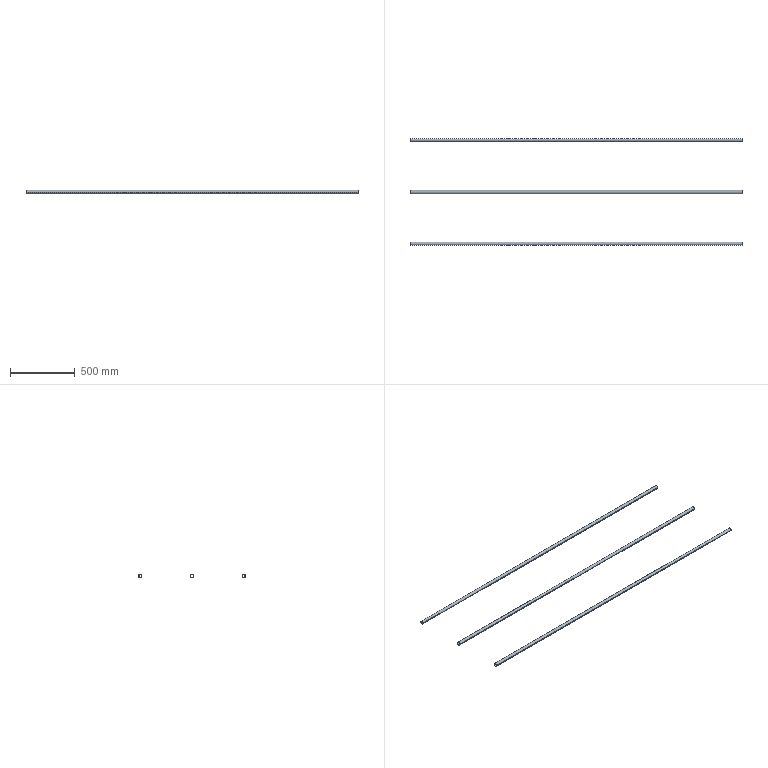Part | STEP file | E3-中转釜护栏2栏杆_Default<As Machined> | 3 solids | 18 faces | box 2560 x 825 x 25 mm | volume 850492 mm3 | cylinder 12 | plane 6 | commonest cylinder face diameters 22 x6 25 x6
STEP:
#1=CARTESIAN_POINT('',(0.,0.,0.));
#2=DIRECTION('',(0.,0.,1.));
#3=DIRECTION('',(1.,0.,0.));
#4=AXIS2_PLACEMENT_3D('',#1,#2,#3);
#5=CARTESIAN_POINT('',(1280.,787.5,0.));
#6=VERTEX_POINT('',#5);
#7=CARTESIAN_POINT('',(1280.,812.5,0.));
#8=VERTEX_POINT('',#7);
#9=CARTESIAN_POINT('',(1280.,800.,0.));
#10=DIRECTION('',(-1.,0.,0.));
#11=DIRECTION('',(0.,1.,0.));
#12=AXIS2_PLACEMENT_3D('',#9,#10,#11);
#13=CIRCLE('',#12,12.5);
#14=CARTESIAN_POINT('',(1280.,800.,0.));
#15=DIRECTION('',(-1.,0.,0.));
#16=DIRECTION('',(0.,-1.,0.));
#17=AXIS2_PLACEMENT_3D('',#14,#15,#16);
#18=CYLINDRICAL_SURFACE('',#17,12.5);
#19=CARTESIAN_POINT('',(-3.142,0.));
#20=DIRECTION('',(1.,0.));
#21=VECTOR('',#20,1.);
#22=LINE('',#19,#21);
#23=(GEOMETRIC_REPRESENTATION_CONTEXT(2)PARAMETRIC_REPRESENTATION_CONTEXT()REPRESENTATION_CONTEXT('',''));
#24=DEFINITIONAL_REPRESENTATION('',(#22),#23);
#25=PCURVE('',#18,#24);
#26=CARTESIAN_POINT('',(1280.,800.,0.));
#27=DIRECTION('',(1.,0.,0.));
#28=DIRECTION('',(0.,1.,0.));
#29=AXIS2_PLACEMENT_3D('',#26,#27,#28);
#30=PLANE('',#29);
#31=CARTESIAN_POINT('',(12.5,0.));
#32=CARTESIAN_POINT('',(12.5,-21.651));
#33=CARTESIAN_POINT('',(-6.25,-10.825));
#34=CARTESIAN_POINT('',(-25.,0.));
#35=CARTESIAN_POINT('',(-6.25,10.825));
#36=CARTESIAN_POINT('',(12.5,21.651));
#37=CARTESIAN_POINT('',(12.5,0.));
#38=(BOUNDED_CURVE()B_SPLINE_CURVE(2,(#31,#32,#33,#34,#35,#36,#37),.UNSPECIFIED.,.T.,.F.)B_SPLINE_CURVE_WITH_KNOTS((1,2,2,2,2,1),(-2.094,0.,2.094,4.189,6.283,8.378),.UNSPECIFIED.)CURVE()GEOMETRIC_REPRESENTATION_ITEM()RATIONAL_B_SPLINE_CURVE((1.,0.5,1.,0.5,1.,0.5,1.))REPRESENTATION_ITEM(''));
#39=(GEOMETRIC_REPRESENTATION_CONTEXT(2)PARAMETRIC_REPRESENTATION_CONTEXT()REPRESENTATION_CONTEXT('',''));
#40=DEFINITIONAL_REPRESENTATION('',(#38),#39);
#41=PCURVE('',#30,#40);
#42=SURFACE_CURVE('',#13,(#25,#41),.PCURVE_S1.);
#43=EDGE_CURVE('',#6,#8,#42,.T.);
#44=ORIENTED_EDGE('',*,*,#43,.T.);
#45=CARTESIAN_POINT('',(-1280.,812.5,0.));
#46=VERTEX_POINT('',#45);
#47=CARTESIAN_POINT('',(1280.,812.5,0.));
#48=DIRECTION('',(-1.,0.,0.));
#49=VECTOR('',#48,1.);
#50=LINE('',#47,#49);
#51=CARTESIAN_POINT('',(3.142,0.));
#52=DIRECTION('',(0.,1.));
#53=VECTOR('',#52,1.);
#54=LINE('',#51,#53);
#55=(GEOMETRIC_REPRESENTATION_CONTEXT(2)PARAMETRIC_REPRESENTATION_CONTEXT()REPRESENTATION_CONTEXT('',''));
#56=DEFINITIONAL_REPRESENTATION('',(#54),#55);
#57=PCURVE('',#18,#56);
#58=CARTESIAN_POINT('',(1280.,800.,0.));
#59=DIRECTION('',(-1.,0.,0.));
#60=DIRECTION('',(0.,-1.,0.));
#61=AXIS2_PLACEMENT_3D('',#58,#59,#60);
#62=CYLINDRICAL_SURFACE('',#61,12.5);
#63=CARTESIAN_POINT('',(3.142,0.));
#64=DIRECTION('',(0.,1.));
#65=VECTOR('',#64,1.);
#66=LINE('',#63,#65);
#67=(GEOMETRIC_REPRESENTATION_CONTEXT(2)PARAMETRIC_REPRESENTATION_CONTEXT()REPRESENTATION_CONTEXT('',''));
#68=DEFINITIONAL_REPRESENTATION('',(#66),#67);
#69=PCURVE('',#62,#68);
#70=SURFACE_CURVE('',#50,(#57,#69),.PCURVE_S1.);
#71=EDGE_CURVE('',#8,#46,#70,.T.);
#72=ORIENTED_EDGE('',*,*,#71,.T.);
#73=CARTESIAN_POINT('',(-1280.,787.5,0.));
#74=VERTEX_POINT('',#73);
#75=CARTESIAN_POINT('',(-1280.,800.,0.));
#76=DIRECTION('',(-1.,0.,0.));
#77=DIRECTION('',(0.,1.,0.));
#78=AXIS2_PLACEMENT_3D('',#75,#76,#77);
#79=CIRCLE('',#78,12.5);
#80=CARTESIAN_POINT('',(-3.142,2560.));
#81=DIRECTION('',(1.,0.));
#82=VECTOR('',#81,1.);
#83=LINE('',#80,#82);
#84=(GEOMETRIC_REPRESENTATION_CONTEXT(2)PARAMETRIC_REPRESENTATION_CONTEXT()REPRESENTATION_CONTEXT('',''));
#85=DEFINITIONAL_REPRESENTATION('',(#83),#84);
#86=PCURVE('',#18,#85);
#87=CARTESIAN_POINT('',(-1280.,800.,0.));
#88=DIRECTION('',(1.,0.,0.));
#89=DIRECTION('',(0.,1.,0.));
#90=AXIS2_PLACEMENT_3D('',#87,#88,#89);
#91=PLANE('',#90);
#92=CARTESIAN_POINT('',(12.5,0.));
#93=CARTESIAN_POINT('',(12.5,-21.651));
#94=CARTESIAN_POINT('',(-6.25,-10.825));
#95=CARTESIAN_POINT('',(-25.,0.));
#96=CARTESIAN_POINT('',(-6.25,10.825));
#97=CARTESIAN_POINT('',(12.5,21.651));
#98=CARTESIAN_POINT('',(12.5,0.));
#99=(BOUNDED_CURVE()B_SPLINE_CURVE(2,(#92,#93,#94,#95,#96,#97,#98),.UNSPECIFIED.,.T.,.F.)B_SPLINE_CURVE_WITH_KNOTS((1,2,2,2,2,1),(-2.094,0.,2.094,4.189,6.283,8.378),.UNSPECIFIED.)CURVE()GEOMETRIC_REPRESENTATION_ITEM()RATIONAL_B_SPLINE_CURVE((1.,0.5,1.,0.5,1.,0.5,1.))REPRESENTATION_ITEM(''));
#100=(GEOMETRIC_REPRESENTATION_CONTEXT(2)PARAMETRIC_REPRESENTATION_CONTEXT()REPRESENTATION_CONTEXT('',''));
#101=DEFINITIONAL_REPRESENTATION('',(#99),#100);
#102=PCURVE('',#91,#101);
#103=SURFACE_CURVE('',#79,(#86,#102),.PCURVE_S1.);
#104=EDGE_CURVE('',#74,#46,#103,.T.);
#105=ORIENTED_EDGE('',*,*,#104,.F.);
#106=CARTESIAN_POINT('',(1280.,787.5,0.));
#107=DIRECTION('',(-1.,0.,0.));
#108=VECTOR('',#107,1.);
#109=LINE('',#106,#108);
#110=CARTESIAN_POINT('',(0.,0.));
#111=DIRECTION('',(0.,1.));
#112=VECTOR('',#111,1.);
#113=LINE('',#110,#112);
#114=(GEOMETRIC_REPRESENTATION_CONTEXT(2)PARAMETRIC_REPRESENTATION_CONTEXT()REPRESENTATION_CONTEXT('',''));
#115=DEFINITIONAL_REPRESENTATION('',(#113),#114);
#116=PCURVE('',#18,#115);
#117=CARTESIAN_POINT('',(6.283,0.));
#118=DIRECTION('',(0.,1.));
#119=VECTOR('',#118,1.);
#120=LINE('',#117,#119);
#121=(GEOMETRIC_REPRESENTATION_CONTEXT(2)PARAMETRIC_REPRESENTATION_CONTEXT()REPRESENTATION_CONTEXT('',''));
#122=DEFINITIONAL_REPRESENTATION('',(#120),#121);
#123=PCURVE('',#62,#122);
#124=SURFACE_CURVE('',#109,(#116,#123),.PCURVE_S1.);
#125=EDGE_CURVE('',#6,#74,#124,.T.);
#126=ORIENTED_EDGE('',*,*,#125,.F.);
#127=EDGE_LOOP('',(#44,#72,#105,#126));
#128=FACE_BOUND('',#127,.T.);
#129=ADVANCED_FACE('',(#128),#18,.T.);
#130=CARTESIAN_POINT('',(1280.,789.,0.));
#131=VERTEX_POINT('',#130);
#132=CARTESIAN_POINT('',(-1280.,789.,0.));
#133=VERTEX_POINT('',#132);
#134=CARTESIAN_POINT('',(1280.,789.,0.));
#135=DIRECTION('',(-1.,0.,0.));
#136=VECTOR('',#135,1.);
#137=LINE('',#134,#136);
#138=CARTESIAN_POINT('',(1280.,800.,0.));
#139=DIRECTION('',(-1.,0.,0.));
#140=DIRECTION('',(0.,-1.,0.));
#141=AXIS2_PLACEMENT_3D('',#138,#139,#140);
#142=CYLINDRICAL_SURFACE('',#141,11.);
#143=CARTESIAN_POINT('',(6.283,0.));
#144=DIRECTION('',(0.,1.));
#145=VECTOR('',#144,1.);
#146=LINE('',#143,#145);
#147=(GEOMETRIC_REPRESENTATION_CONTEXT(2)PARAMETRIC_REPRESENTATION_CONTEXT()REPRESENTATION_CONTEXT('',''));
#148=DEFINITIONAL_REPRESENTATION('',(#146),#147);
#149=PCURVE('',#142,#148);
#150=CARTESIAN_POINT('',(1280.,800.,0.));
#151=DIRECTION('',(-1.,0.,0.));
#152=DIRECTION('',(0.,-1.,0.));
#153=AXIS2_PLACEMENT_3D('',#150,#151,#152);
#154=CYLINDRICAL_SURFACE('',#153,11.);
#155=CARTESIAN_POINT('',(0.,0.));
#156=DIRECTION('',(0.,1.));
#157=VECTOR('',#156,1.);
#158=LINE('',#155,#157);
#159=(GEOMETRIC_REPRESENTATION_CONTEXT(2)PARAMETRIC_REPRESENTATION_CONTEXT()REPRESENTATION_CONTEXT('',''));
#160=DEFINITIONAL_REPRESENTATION('',(#158),#159);
#161=PCURVE('',#154,#160);
#162=SURFACE_CURVE('',#137,(#149,#161),.PCURVE_S1.);
#163=EDGE_CURVE('',#131,#133,#162,.T.);
#164=ORIENTED_EDGE('',*,*,#163,.T.);
#165=CARTESIAN_POINT('',(-1280.,811.,0.));
#166=VERTEX_POINT('',#165);
#167=CARTESIAN_POINT('',(-1280.,800.,0.));
#168=DIRECTION('',(-1.,0.,0.));
#169=DIRECTION('',(0.,1.,0.));
#170=AXIS2_PLACEMENT_3D('',#167,#168,#169);
#171=CIRCLE('',#170,11.);
#172=CARTESIAN_POINT('',(3.142,2560.));
#173=DIRECTION('',(1.,0.));
#174=VECTOR('',#173,1.);
#175=LINE('',#172,#174);
#176=(GEOMETRIC_REPRESENTATION_CONTEXT(2)PARAMETRIC_REPRESENTATION_CONTEXT()REPRESENTATION_CONTEXT('',''));
#177=DEFINITIONAL_REPRESENTATION('',(#175),#176);
#178=PCURVE('',#142,#177);
#179=CARTESIAN_POINT('',(11.,0.));
#180=CARTESIAN_POINT('',(11.,-19.053));
#181=CARTESIAN_POINT('',(-5.5,-9.526));
#182=CARTESIAN_POINT('',(-22.,0.));
#183=CARTESIAN_POINT('',(-5.5,9.526));
#184=CARTESIAN_POINT('',(11.,19.053));
#185=CARTESIAN_POINT('',(11.,0.));
#186=(BOUNDED_CURVE()B_SPLINE_CURVE(2,(#179,#180,#181,#182,#183,#184,#185),.UNSPECIFIED.,.T.,.F.)B_SPLINE_CURVE_WITH_KNOTS((1,2,2,2,2,1),(-2.094,0.,2.094,4.189,6.283,8.378),.UNSPECIFIED.)CURVE()GEOMETRIC_REPRESENTATION_ITEM()RATIONAL_B_SPLINE_CURVE((1.,0.5,1.,0.5,1.,0.5,1.))REPRESENTATION_ITEM(''));
#187=(GEOMETRIC_REPRESENTATION_CONTEXT(2)PARAMETRIC_REPRESENTATION_CONTEXT()REPRESENTATION_CONTEXT('',''));
#188=DEFINITIONAL_REPRESENTATION('',(#186),#187);
#189=PCURVE('',#91,#188);
#190=SURFACE_CURVE('',#171,(#178,#189),.PCURVE_S1.);
#191=EDGE_CURVE('',#166,#133,#190,.T.);
#192=ORIENTED_EDGE('',*,*,#191,.F.);
#193=CARTESIAN_POINT('',(1280.,811.,0.));
#194=VERTEX_POINT('',#193);
#195=CARTESIAN_POINT('',(1280.,811.,0.));
#196=DIRECTION('',(-1.,0.,0.));
#197=VECTOR('',#196,1.);
#198=LINE('',#195,#197);
#199=CARTESIAN_POINT('',(3.142,0.));
#200=DIRECTION('',(0.,1.));
#201=VECTOR('',#200,1.);
#202=LINE('',#199,#201);
#203=(GEOMETRIC_REPRESENTATION_CONTEXT(2)PARAMETRIC_REPRESENTATION_CONTEXT()REPRESENTATION_CONTEXT('',''));
#204=DEFINITIONAL_REPRESENTATION('',(#202),#203);
#205=PCURVE('',#142,#204);
#206=CARTESIAN_POINT('',(3.142,0.));
#207=DIRECTION('',(0.,1.));
#208=VECTOR('',#207,1.);
#209=LINE('',#206,#208);
#210=(GEOMETRIC_REPRESENTATION_CONTEXT(2)PARAMETRIC_REPRESENTATION_CONTEXT()REPRESENTATION_CONTEXT('',''));
#211=DEFINITIONAL_REPRESENTATION('',(#209),#210);
#212=PCURVE('',#154,#211);
#213=SURFACE_CURVE('',#198,(#205,#212),.PCURVE_S1.);
#214=EDGE_CURVE('',#194,#166,#213,.T.);
#215=ORIENTED_EDGE('',*,*,#214,.F.);
#216=CARTESIAN_POINT('',(1280.,800.,0.));
#217=DIRECTION('',(-1.,0.,0.));
#218=DIRECTION('',(0.,1.,0.));
#219=AXIS2_PLACEMENT_3D('',#216,#217,#218);
#220=CIRCLE('',#219,11.);
#221=CARTESIAN_POINT('',(3.142,0.));
#222=DIRECTION('',(1.,0.));
#223=VECTOR('',#222,1.);
#224=LINE('',#221,#223);
#225=(GEOMETRIC_REPRESENTATION_CONTEXT(2)PARAMETRIC_REPRESENTATION_CONTEXT()REPRESENTATION_CONTEXT('',''));
#226=DEFINITIONAL_REPRESENTATION('',(#224),#225);
#227=PCURVE('',#142,#226);
#228=CARTESIAN_POINT('',(11.,0.));
#229=CARTESIAN_POINT('',(11.,-19.053));
#230=CARTESIAN_POINT('',(-5.5,-9.526));
#231=CARTESIAN_POINT('',(-22.,0.));
#232=CARTESIAN_POINT('',(-5.5,9.526));
#233=CARTESIAN_POINT('',(11.,19.053));
#234=CARTESIAN_POINT('',(11.,0.));
#235=(BOUNDED_CURVE()B_SPLINE_CURVE(2,(#228,#229,#230,#231,#232,#233,#234),.UNSPECIFIED.,.T.,.F.)B_SPLINE_CURVE_WITH_KNOTS((1,2,2,2,2,1),(-2.094,0.,2.094,4.189,6.283,8.378),.UNSPECIFIED.)CURVE()GEOMETRIC_REPRESENTATION_ITEM()RATIONAL_B_SPLINE_CURVE((1.,0.5,1.,0.5,1.,0.5,1.))REPRESENTATION_ITEM(''));
#236=(GEOMETRIC_REPRESENTATION_CONTEXT(2)PARAMETRIC_REPRESENTATION_CONTEXT()REPRESENTATION_CONTEXT('',''));
#237=DEFINITIONAL_REPRESENTATION('',(#235),#236);
#238=PCURVE('',#30,#237);
#239=SURFACE_CURVE('',#220,(#227,#238),.PCURVE_S1.);
#240=EDGE_CURVE('',#194,#131,#239,.T.);
#241=ORIENTED_EDGE('',*,*,#240,.T.);
#242=EDGE_LOOP('',(#164,#192,#215,#241));
#243=FACE_BOUND('',#242,.F.);
#244=ADVANCED_FACE('',(#243),#142,.F.);
#245=CARTESIAN_POINT('',(-1280.,800.,0.));
#246=DIRECTION('',(-1.,0.,0.));
#247=DIRECTION('',(0.,1.,0.));
#248=AXIS2_PLACEMENT_3D('',#245,#246,#247);
#249=CIRCLE('',#248,11.);
#250=CARTESIAN_POINT('',(-3.142,2560.));
#251=DIRECTION('',(1.,0.));
#252=VECTOR('',#251,1.);
#253=LINE('',#250,#252);
#254=(GEOMETRIC_REPRESENTATION_CONTEXT(2)PARAMETRIC_REPRESENTATION_CONTEXT()REPRESENTATION_CONTEXT('',''));
#255=DEFINITIONAL_REPRESENTATION('',(#253),#254);
#256=PCURVE('',#154,#255);
#257=CARTESIAN_POINT('',(11.,0.));
#258=CARTESIAN_POINT('',(11.,-19.053));
#259=CARTESIAN_POINT('',(-5.5,-9.526));
#260=CARTESIAN_POINT('',(-22.,0.));
#261=CARTESIAN_POINT('',(-5.5,9.526));
#262=CARTESIAN_POINT('',(11.,19.053));
#263=CARTESIAN_POINT('',(11.,0.));
#264=(BOUNDED_CURVE()B_SPLINE_CURVE(2,(#257,#258,#259,#260,#261,#262,#263),.UNSPECIFIED.,.T.,.F.)B_SPLINE_CURVE_WITH_KNOTS((1,2,2,2,2,1),(-2.094,0.,2.094,4.189,6.283,8.378),.UNSPECIFIED.)CURVE()GEOMETRIC_REPRESENTATION_ITEM()RATIONAL_B_SPLINE_CURVE((1.,0.5,1.,0.5,1.,0.5,1.))REPRESENTATION_ITEM(''));
#265=(GEOMETRIC_REPRESENTATION_CONTEXT(2)PARAMETRIC_REPRESENTATION_CONTEXT()REPRESENTATION_CONTEXT('',''));
#266=DEFINITIONAL_REPRESENTATION('',(#264),#265);
#267=PCURVE('',#91,#266);
#268=SURFACE_CURVE('',#249,(#256,#267),.PCURVE_S1.);
#269=EDGE_CURVE('',#133,#166,#268,.T.);
#270=ORIENTED_EDGE('',*,*,#269,.F.);
#271=ORIENTED_EDGE('',*,*,#163,.F.);
#272=CARTESIAN_POINT('',(1280.,800.,0.));
#273=DIRECTION('',(-1.,0.,0.));
#274=DIRECTION('',(0.,1.,0.));
#275=AXIS2_PLACEMENT_3D('',#272,#273,#274);
#276=CIRCLE('',#275,11.);
#277=CARTESIAN_POINT('',(-3.142,0.));
#278=DIRECTION('',(1.,0.));
#279=VECTOR('',#278,1.);
#280=LINE('',#277,#279);
#281=(GEOMETRIC_REPRESENTATION_CONTEXT(2)PARAMETRIC_REPRESENTATION_CONTEXT()REPRESENTATION_CONTEXT('',''));
#282=DEFINITIONAL_REPRESENTATION('',(#280),#281);
#283=PCURVE('',#154,#282);
#284=CARTESIAN_POINT('',(11.,0.));
#285=CARTESIAN_POINT('',(11.,-19.053));
#286=CARTESIAN_POINT('',(-5.5,-9.526));
#287=CARTESIAN_POINT('',(-22.,0.));
#288=CARTESIAN_POINT('',(-5.5,9.526));
#289=CARTESIAN_POINT('',(11.,19.053));
#290=CARTESIAN_POINT('',(11.,0.));
#291=(BOUNDED_CURVE()B_SPLINE_CURVE(2,(#284,#285,#286,#287,#288,#289,#290),.UNSPECIFIED.,.T.,.F.)B_SPLINE_CURVE_WITH_KNOTS((1,2,2,2,2,1),(-2.094,0.,2.094,4.189,6.283,8.378),.UNSPECIFIED.)CURVE()GEOMETRIC_REPRESENTATION_ITEM()RATIONAL_B_SPLINE_CURVE((1.,0.5,1.,0.5,1.,0.5,1.))REPRESENTATION_ITEM(''));
#292=(GEOMETRIC_REPRESENTATION_CONTEXT(2)PARAMETRIC_REPRESENTATION_CONTEXT()REPRESENTATION_CONTEXT('',''));
#293=DEFINITIONAL_REPRESENTATION('',(#291),#292);
#294=PCURVE('',#30,#293);
#295=SURFACE_CURVE('',#276,(#283,#294),.PCURVE_S1.);
#296=EDGE_CURVE('',#131,#194,#295,.T.);
#297=ORIENTED_EDGE('',*,*,#296,.T.);
#298=ORIENTED_EDGE('',*,*,#214,.T.);
#299=EDGE_LOOP('',(#270,#271,#297,#298));
#300=FACE_BOUND('',#299,.F.);
#301=ADVANCED_FACE('',(#300),#154,.F.);
#302=ORIENTED_EDGE('',*,*,#71,.F.);
#303=CARTESIAN_POINT('',(1280.,800.,0.));
#304=DIRECTION('',(-1.,0.,0.));
#305=DIRECTION('',(0.,1.,0.));
#306=AXIS2_PLACEMENT_3D('',#303,#304,#305);
#307=CIRCLE('',#306,12.5);
#308=CARTESIAN_POINT('',(3.142,0.));
#309=DIRECTION('',(1.,0.));
#310=VECTOR('',#309,1.);
#311=LINE('',#308,#310);
#312=(GEOMETRIC_REPRESENTATION_CONTEXT(2)PARAMETRIC_REPRESENTATION_CONTEXT()REPRESENTATION_CONTEXT('',''));
#313=DEFINITIONAL_REPRESENTATION('',(#311),#312);
#314=PCURVE('',#62,#313);
#315=CARTESIAN_POINT('',(12.5,0.));
#316=CARTESIAN_POINT('',(12.5,-21.651));
#317=CARTESIAN_POINT('',(-6.25,-10.825));
#318=CARTESIAN_POINT('',(-25.,0.));
#319=CARTESIAN_POINT('',(-6.25,10.825));
#320=CARTESIAN_POINT('',(12.5,21.651));
#321=CARTESIAN_POINT('',(12.5,0.));
#322=(BOUNDED_CURVE()B_SPLINE_CURVE(2,(#315,#316,#317,#318,#319,#320,#321),.UNSPECIFIED.,.T.,.F.)B_SPLINE_CURVE_WITH_KNOTS((1,2,2,2,2,1),(-2.094,0.,2.094,4.189,6.283,8.378),.UNSPECIFIED.)CURVE()GEOMETRIC_REPRESENTATION_ITEM()RATIONAL_B_SPLINE_CURVE((1.,0.5,1.,0.5,1.,0.5,1.))REPRESENTATION_ITEM(''));
#323=(GEOMETRIC_REPRESENTATION_CONTEXT(2)PARAMETRIC_REPRESENTATION_CONTEXT()REPRESENTATION_CONTEXT('',''));
#324=DEFINITIONAL_REPRESENTATION('',(#322),#323);
#325=PCURVE('',#30,#324);
#326=SURFACE_CURVE('',#307,(#314,#325),.PCURVE_S1.);
#327=EDGE_CURVE('',#8,#6,#326,.T.);
#328=ORIENTED_EDGE('',*,*,#327,.T.);
#329=ORIENTED_EDGE('',*,*,#125,.T.);
#330=CARTESIAN_POINT('',(-1280.,800.,0.));
#331=DIRECTION('',(-1.,0.,0.));
#332=DIRECTION('',(0.,1.,0.));
#333=AXIS2_PLACEMENT_3D('',#330,#331,#332);
#334=CIRCLE('',#333,12.5);
#335=CARTESIAN_POINT('',(3.142,2560.));
#336=DIRECTION('',(1.,0.));
#337=VECTOR('',#336,1.);
#338=LINE('',#335,#337);
#339=(GEOMETRIC_REPRESENTATION_CONTEXT(2)PARAMETRIC_REPRESENTATION_CONTEXT()REPRESENTATION_CONTEXT('',''));
#340=DEFINITIONAL_REPRESENTATION('',(#338),#339);
#341=PCURVE('',#62,#340);
#342=CARTESIAN_POINT('',(12.5,0.));
#343=CARTESIAN_POINT('',(12.5,-21.651));
#344=CARTESIAN_POINT('',(-6.25,-10.825));
#345=CARTESIAN_POINT('',(-25.,0.));
#346=CARTESIAN_POINT('',(-6.25,10.825));
#347=CARTESIAN_POINT('',(12.5,21.651));
#348=CARTESIAN_POINT('',(12.5,0.));
#349=(BOUNDED_CURVE()B_SPLINE_CURVE(2,(#342,#343,#344,#345,#346,#347,#348),.UNSPECIFIED.,.T.,.F.)B_SPLINE_CURVE_WITH_KNOTS((1,2,2,2,2,1),(-2.094,0.,2.094,4.189,6.283,8.378),.UNSPECIFIED.)CURVE()GEOMETRIC_REPRESENTATION_ITEM()RATIONAL_B_SPLINE_CURVE((1.,0.5,1.,0.5,1.,0.5,1.))REPRESENTATION_ITEM(''));
#350=(GEOMETRIC_REPRESENTATION_CONTEXT(2)PARAMETRIC_REPRESENTATION_CONTEXT()REPRESENTATION_CONTEXT('',''));
#351=DEFINITIONAL_REPRESENTATION('',(#349),#350);
#352=PCURVE('',#91,#351);
#353=SURFACE_CURVE('',#334,(#341,#352),.PCURVE_S1.);
#354=EDGE_CURVE('',#46,#74,#353,.T.);
#355=ORIENTED_EDGE('',*,*,#354,.F.);
#356=EDGE_LOOP('',(#302,#328,#329,#355));
#357=FACE_BOUND('',#356,.T.);
#358=ADVANCED_FACE('',(#357),#62,.T.);
#359=ORIENTED_EDGE('',*,*,#296,.T.);
#360=ORIENTED_EDGE('',*,*,#240,.T.);
#361=EDGE_LOOP('',(#359,#360));
#362=FACE_BOUND('',#361,.T.);
#363=ORIENTED_EDGE('',*,*,#43,.F.);
#364=ORIENTED_EDGE('',*,*,#327,.F.);
#365=EDGE_LOOP('',(#363,#364));
#366=FACE_BOUND('',#365,.T.);
#367=ADVANCED_FACE('',(#362,#366),#30,.T.);
#368=ORIENTED_EDGE('',*,*,#269,.F.);
#369=ORIENTED_EDGE('',*,*,#191,.F.);
#370=EDGE_LOOP('',(#368,#369));
#371=FACE_BOUND('',#370,.T.);
#372=ORIENTED_EDGE('',*,*,#104,.T.);
#373=ORIENTED_EDGE('',*,*,#354,.T.);
#374=EDGE_LOOP('',(#372,#373));
#375=FACE_BOUND('',#374,.T.);
#376=ADVANCED_FACE('',(#371,#375),#91,.F.);
#377=CLOSED_SHELL('',(#129,#244,#301,#358,#367,#376));
#378=MANIFOLD_SOLID_BREP('',#377);
#379=CARTESIAN_POINT('',(1280.,-12.5,0.));
#380=VERTEX_POINT('',#379);
#381=CARTESIAN_POINT('',(1280.,12.5,0.));
#382=VERTEX_POINT('',#381);
#383=CARTESIAN_POINT('',(1280.,0.,0.));
#384=DIRECTION('',(-1.,0.,0.));
#385=DIRECTION('',(0.,1.,0.));
#386=AXIS2_PLACEMENT_3D('',#383,#384,#385);
#387=CIRCLE('',#386,12.5);
#388=CARTESIAN_POINT('',(1280.,0.,0.));
#389=DIRECTION('',(-1.,0.,0.));
#390=DIRECTION('',(0.,-1.,0.));
#391=AXIS2_PLACEMENT_3D('',#388,#389,#390);
#392=CYLINDRICAL_SURFACE('',#391,12.5);
#393=CARTESIAN_POINT('',(-3.142,0.));
#394=DIRECTION('',(1.,0.));
#395=VECTOR('',#394,1.);
#396=LINE('',#393,#395);
#397=(GEOMETRIC_REPRESENTATION_CONTEXT(2)PARAMETRIC_REPRESENTATION_CONTEXT()REPRESENTATION_CONTEXT('',''));
#398=DEFINITIONAL_REPRESENTATION('',(#396),#397);
#399=PCURVE('',#392,#398);
#400=CARTESIAN_POINT('',(1280.,0.,0.));
#401=DIRECTION('',(1.,0.,0.));
#402=DIRECTION('',(0.,1.,0.));
#403=AXIS2_PLACEMENT_3D('',#400,#401,#402);
#404=PLANE('',#403);
#405=CARTESIAN_POINT('',(12.5,0.));
#406=CARTESIAN_POINT('',(12.5,-21.651));
#407=CARTESIAN_POINT('',(-6.25,-10.825));
#408=CARTESIAN_POINT('',(-25.,0.));
#409=CARTESIAN_POINT('',(-6.25,10.825));
#410=CARTESIAN_POINT('',(12.5,21.651));
#411=CARTESIAN_POINT('',(12.5,0.));
#412=(BOUNDED_CURVE()B_SPLINE_CURVE(2,(#405,#406,#407,#408,#409,#410,#411),.UNSPECIFIED.,.T.,.F.)B_SPLINE_CURVE_WITH_KNOTS((1,2,2,2,2,1),(-2.094,0.,2.094,4.189,6.283,8.378),.UNSPECIFIED.)CURVE()GEOMETRIC_REPRESENTATION_ITEM()RATIONAL_B_SPLINE_CURVE((1.,0.5,1.,0.5,1.,0.5,1.))REPRESENTATION_ITEM(''));
#413=(GEOMETRIC_REPRESENTATION_CONTEXT(2)PARAMETRIC_REPRESENTATION_CONTEXT()REPRESENTATION_CONTEXT('',''));
#414=DEFINITIONAL_REPRESENTATION('',(#412),#413);
#415=PCURVE('',#404,#414);
#416=SURFACE_CURVE('',#387,(#399,#415),.PCURVE_S1.);
#417=EDGE_CURVE('',#380,#382,#416,.T.);
#418=ORIENTED_EDGE('',*,*,#417,.T.);
#419=CARTESIAN_POINT('',(-1280.,12.5,0.));
#420=VERTEX_POINT('',#419);
#421=CARTESIAN_POINT('',(1280.,12.5,0.));
#422=DIRECTION('',(-1.,0.,0.));
#423=VECTOR('',#422,1.);
#424=LINE('',#421,#423);
#425=CARTESIAN_POINT('',(3.142,0.));
#426=DIRECTION('',(0.,1.));
#427=VECTOR('',#426,1.);
#428=LINE('',#425,#427);
#429=(GEOMETRIC_REPRESENTATION_CONTEXT(2)PARAMETRIC_REPRESENTATION_CONTEXT()REPRESENTATION_CONTEXT('',''));
#430=DEFINITIONAL_REPRESENTATION('',(#428),#429);
#431=PCURVE('',#392,#430);
#432=CARTESIAN_POINT('',(1280.,0.,0.));
#433=DIRECTION('',(-1.,0.,0.));
#434=DIRECTION('',(0.,-1.,0.));
#435=AXIS2_PLACEMENT_3D('',#432,#433,#434);
#436=CYLINDRICAL_SURFACE('',#435,12.5);
#437=CARTESIAN_POINT('',(3.142,0.));
#438=DIRECTION('',(0.,1.));
#439=VECTOR('',#438,1.);
#440=LINE('',#437,#439);
#441=(GEOMETRIC_REPRESENTATION_CONTEXT(2)PARAMETRIC_REPRESENTATION_CONTEXT()REPRESENTATION_CONTEXT('',''));
#442=DEFINITIONAL_REPRESENTATION('',(#440),#441);
#443=PCURVE('',#436,#442);
#444=SURFACE_CURVE('',#424,(#431,#443),.PCURVE_S1.);
#445=EDGE_CURVE('',#382,#420,#444,.T.);
#446=ORIENTED_EDGE('',*,*,#445,.T.);
#447=CARTESIAN_POINT('',(-1280.,-12.5,0.));
#448=VERTEX_POINT('',#447);
#449=CARTESIAN_POINT('',(-1280.,0.,0.));
#450=DIRECTION('',(-1.,0.,0.));
#451=DIRECTION('',(0.,1.,0.));
#452=AXIS2_PLACEMENT_3D('',#449,#450,#451);
#453=CIRCLE('',#452,12.5);
#454=CARTESIAN_POINT('',(-3.142,2560.));
#455=DIRECTION('',(1.,0.));
#456=VECTOR('',#455,1.);
#457=LINE('',#454,#456);
#458=(GEOMETRIC_REPRESENTATION_CONTEXT(2)PARAMETRIC_REPRESENTATION_CONTEXT()REPRESENTATION_CONTEXT('',''));
#459=DEFINITIONAL_REPRESENTATION('',(#457),#458);
#460=PCURVE('',#392,#459);
#461=CARTESIAN_POINT('',(-1280.,0.,0.));
#462=DIRECTION('',(1.,0.,0.));
#463=DIRECTION('',(0.,1.,0.));
#464=AXIS2_PLACEMENT_3D('',#461,#462,#463);
#465=PLANE('',#464);
#466=CARTESIAN_POINT('',(12.5,0.));
#467=CARTESIAN_POINT('',(12.5,-21.651));
#468=CARTESIAN_POINT('',(-6.25,-10.825));
#469=CARTESIAN_POINT('',(-25.,0.));
#470=CARTESIAN_POINT('',(-6.25,10.825));
#471=CARTESIAN_POINT('',(12.5,21.651));
#472=CARTESIAN_POINT('',(12.5,0.));
#473=(BOUNDED_CURVE()B_SPLINE_CURVE(2,(#466,#467,#468,#469,#470,#471,#472),.UNSPECIFIED.,.T.,.F.)B_SPLINE_CURVE_WITH_KNOTS((1,2,2,2,2,1),(-2.094,0.,2.094,4.189,6.283,8.378),.UNSPECIFIED.)CURVE()GEOMETRIC_REPRESENTATION_ITEM()RATIONAL_B_SPLINE_CURVE((1.,0.5,1.,0.5,1.,0.5,1.))REPRESENTATION_ITEM(''));
#474=(GEOMETRIC_REPRESENTATION_CONTEXT(2)PARAMETRIC_REPRESENTATION_CONTEXT()REPRESENTATION_CONTEXT('',''));
#475=DEFINITIONAL_REPRESENTATION('',(#473),#474);
#476=PCURVE('',#465,#475);
#477=SURFACE_CURVE('',#453,(#460,#476),.PCURVE_S1.);
#478=EDGE_CURVE('',#448,#420,#477,.T.);
#479=ORIENTED_EDGE('',*,*,#478,.F.);
#480=CARTESIAN_POINT('',(1280.,-12.5,0.));
#481=DIRECTION('',(-1.,0.,0.));
#482=VECTOR('',#481,1.);
#483=LINE('',#480,#482);
#484=CARTESIAN_POINT('',(0.,0.));
#485=DIRECTION('',(0.,1.));
#486=VECTOR('',#485,1.);
#487=LINE('',#484,#486);
#488=(GEOMETRIC_REPRESENTATION_CONTEXT(2)PARAMETRIC_REPRESENTATION_CONTEXT()REPRESENTATION_CONTEXT('',''));
#489=DEFINITIONAL_REPRESENTATION('',(#487),#488);
#490=PCURVE('',#392,#489);
#491=CARTESIAN_POINT('',(6.283,0.));
#492=DIRECTION('',(0.,1.));
#493=VECTOR('',#492,1.);
#494=LINE('',#491,#493);
#495=(GEOMETRIC_REPRESENTATION_CONTEXT(2)PARAMETRIC_REPRESENTATION_CONTEXT()REPRESENTATION_CONTEXT('',''));
#496=DEFINITIONAL_REPRESENTATION('',(#494),#495);
#497=PCURVE('',#436,#496);
#498=SURFACE_CURVE('',#483,(#490,#497),.PCURVE_S1.);
#499=EDGE_CURVE('',#380,#448,#498,.T.);
#500=ORIENTED_EDGE('',*,*,#499,.F.);
#501=EDGE_LOOP('',(#418,#446,#479,#500));
#502=FACE_BOUND('',#501,.T.);
#503=ADVANCED_FACE('',(#502),#392,.T.);
#504=CARTESIAN_POINT('',(1280.,-11.,0.));
#505=VERTEX_POINT('',#504);
#506=CARTESIAN_POINT('',(-1280.,-11.,0.));
#507=VERTEX_POINT('',#506);
#508=CARTESIAN_POINT('',(1280.,-11.,0.));
#509=DIRECTION('',(-1.,0.,0.));
#510=VECTOR('',#509,1.);
#511=LINE('',#508,#510);
#512=CARTESIAN_POINT('',(1280.,0.,0.));
#513=DIRECTION('',(-1.,0.,0.));
#514=DIRECTION('',(0.,-1.,0.));
#515=AXIS2_PLACEMENT_3D('',#512,#513,#514);
#516=CYLINDRICAL_SURFACE('',#515,11.);
#517=CARTESIAN_POINT('',(6.283,0.));
#518=DIRECTION('',(0.,1.));
#519=VECTOR('',#518,1.);
#520=LINE('',#517,#519);
#521=(GEOMETRIC_REPRESENTATION_CONTEXT(2)PARAMETRIC_REPRESENTATION_CONTEXT()REPRESENTATION_CONTEXT('',''));
#522=DEFINITIONAL_REPRESENTATION('',(#520),#521);
#523=PCURVE('',#516,#522);
#524=CARTESIAN_POINT('',(1280.,0.,0.));
#525=DIRECTION('',(-1.,0.,0.));
#526=DIRECTION('',(0.,-1.,0.));
#527=AXIS2_PLACEMENT_3D('',#524,#525,#526);
#528=CYLINDRICAL_SURFACE('',#527,11.);
#529=CARTESIAN_POINT('',(0.,0.));
#530=DIRECTION('',(0.,1.));
#531=VECTOR('',#530,1.);
#532=LINE('',#529,#531);
#533=(GEOMETRIC_REPRESENTATION_CONTEXT(2)PARAMETRIC_REPRESENTATION_CONTEXT()REPRESENTATION_CONTEXT('',''));
#534=DEFINITIONAL_REPRESENTATION('',(#532),#533);
#535=PCURVE('',#528,#534);
#536=SURFACE_CURVE('',#511,(#523,#535),.PCURVE_S1.);
#537=EDGE_CURVE('',#505,#507,#536,.T.);
#538=ORIENTED_EDGE('',*,*,#537,.T.);
#539=CARTESIAN_POINT('',(-1280.,11.,0.));
#540=VERTEX_POINT('',#539);
#541=CARTESIAN_POINT('',(-1280.,0.,0.));
#542=DIRECTION('',(-1.,0.,0.));
#543=DIRECTION('',(0.,1.,0.));
#544=AXIS2_PLACEMENT_3D('',#541,#542,#543);
#545=CIRCLE('',#544,11.);
#546=CARTESIAN_POINT('',(3.142,2560.));
#547=DIRECTION('',(1.,0.));
#548=VECTOR('',#547,1.);
#549=LINE('',#546,#548);
#550=(GEOMETRIC_REPRESENTATION_CONTEXT(2)PARAMETRIC_REPRESENTATION_CONTEXT()REPRESENTATION_CONTEXT('',''));
#551=DEFINITIONAL_REPRESENTATION('',(#549),#550);
#552=PCURVE('',#516,#551);
#553=CARTESIAN_POINT('',(11.,0.));
#554=CARTESIAN_POINT('',(11.,-19.053));
#555=CARTESIAN_POINT('',(-5.5,-9.526));
#556=CARTESIAN_POINT('',(-22.,0.));
#557=CARTESIAN_POINT('',(-5.5,9.526));
#558=CARTESIAN_POINT('',(11.,19.053));
#559=CARTESIAN_POINT('',(11.,0.));
#560=(BOUNDED_CURVE()B_SPLINE_CURVE(2,(#553,#554,#555,#556,#557,#558,#559),.UNSPECIFIED.,.T.,.F.)B_SPLINE_CURVE_WITH_KNOTS((1,2,2,2,2,1),(-2.094,0.,2.094,4.189,6.283,8.378),.UNSPECIFIED.)CURVE()GEOMETRIC_REPRESENTATION_ITEM()RATIONAL_B_SPLINE_CURVE((1.,0.5,1.,0.5,1.,0.5,1.))REPRESENTATION_ITEM(''));
#561=(GEOMETRIC_REPRESENTATION_CONTEXT(2)PARAMETRIC_REPRESENTATION_CONTEXT()REPRESENTATION_CONTEXT('',''));
#562=DEFINITIONAL_REPRESENTATION('',(#560),#561);
#563=PCURVE('',#465,#562);
#564=SURFACE_CURVE('',#545,(#552,#563),.PCURVE_S1.);
#565=EDGE_CURVE('',#540,#507,#564,.T.);
#566=ORIENTED_EDGE('',*,*,#565,.F.);
#567=CARTESIAN_POINT('',(1280.,11.,0.));
#568=VERTEX_POINT('',#567);
#569=CARTESIAN_POINT('',(1280.,11.,0.));
#570=DIRECTION('',(-1.,0.,0.));
#571=VECTOR('',#570,1.);
#572=LINE('',#569,#571);
#573=CARTESIAN_POINT('',(3.142,0.));
#574=DIRECTION('',(0.,1.));
#575=VECTOR('',#574,1.);
#576=LINE('',#573,#575);
#577=(GEOMETRIC_REPRESENTATION_CONTEXT(2)PARAMETRIC_REPRESENTATION_CONTEXT()REPRESENTATION_CONTEXT('',''));
#578=DEFINITIONAL_REPRESENTATION('',(#576),#577);
#579=PCURVE('',#516,#578);
#580=CARTESIAN_POINT('',(3.142,0.));
#581=DIRECTION('',(0.,1.));
#582=VECTOR('',#581,1.);
#583=LINE('',#580,#582);
#584=(GEOMETRIC_REPRESENTATION_CONTEXT(2)PARAMETRIC_REPRESENTATION_CONTEXT()REPRESENTATION_CONTEXT('',''));
#585=DEFINITIONAL_REPRESENTATION('',(#583),#584);
#586=PCURVE('',#528,#585);
#587=SURFACE_CURVE('',#572,(#579,#586),.PCURVE_S1.);
#588=EDGE_CURVE('',#568,#540,#587,.T.);
#589=ORIENTED_EDGE('',*,*,#588,.F.);
#590=CARTESIAN_POINT('',(1280.,0.,0.));
#591=DIRECTION('',(-1.,0.,0.));
#592=DIRECTION('',(0.,1.,0.));
#593=AXIS2_PLACEMENT_3D('',#590,#591,#592);
#594=CIRCLE('',#593,11.);
#595=CARTESIAN_POINT('',(3.142,0.));
#596=DIRECTION('',(1.,0.));
#597=VECTOR('',#596,1.);
#598=LINE('',#595,#597);
#599=(GEOMETRIC_REPRESENTATION_CONTEXT(2)PARAMETRIC_REPRESENTATION_CONTEXT()REPRESENTATION_CONTEXT('',''));
#600=DEFINITIONAL_REPRESENTATION('',(#598),#599);
#601=PCURVE('',#516,#600);
#602=CARTESIAN_POINT('',(11.,0.));
#603=CARTESIAN_POINT('',(11.,-19.053));
#604=CARTESIAN_POINT('',(-5.5,-9.526));
#605=CARTESIAN_POINT('',(-22.,0.));
#606=CARTESIAN_POINT('',(-5.5,9.526));
#607=CARTESIAN_POINT('',(11.,19.053));
#608=CARTESIAN_POINT('',(11.,0.));
#609=(BOUNDED_CURVE()B_SPLINE_CURVE(2,(#602,#603,#604,#605,#606,#607,#608),.UNSPECIFIED.,.T.,.F.)B_SPLINE_CURVE_WITH_KNOTS((1,2,2,2,2,1),(-2.094,0.,2.094,4.189,6.283,8.378),.UNSPECIFIED.)CURVE()GEOMETRIC_REPRESENTATION_ITEM()RATIONAL_B_SPLINE_CURVE((1.,0.5,1.,0.5,1.,0.5,1.))REPRESENTATION_ITEM(''));
#610=(GEOMETRIC_REPRESENTATION_CONTEXT(2)PARAMETRIC_REPRESENTATION_CONTEXT()REPRESENTATION_CONTEXT('',''));
#611=DEFINITIONAL_REPRESENTATION('',(#609),#610);
#612=PCURVE('',#404,#611);
#613=SURFACE_CURVE('',#594,(#601,#612),.PCURVE_S1.);
#614=EDGE_CURVE('',#568,#505,#613,.T.);
#615=ORIENTED_EDGE('',*,*,#614,.T.);
#616=EDGE_LOOP('',(#538,#566,#589,#615));
#617=FACE_BOUND('',#616,.F.);
#618=ADVANCED_FACE('',(#617),#516,.F.);
#619=CARTESIAN_POINT('',(-1280.,0.,0.));
#620=DIRECTION('',(-1.,0.,0.));
#621=DIRECTION('',(0.,1.,0.));
#622=AXIS2_PLACEMENT_3D('',#619,#620,#621);
#623=CIRCLE('',#622,11.);
#624=CARTESIAN_POINT('',(-3.142,2560.));
#625=DIRECTION('',(1.,0.));
#626=VECTOR('',#625,1.);
#627=LINE('',#624,#626);
#628=(GEOMETRIC_REPRESENTATION_CONTEXT(2)PARAMETRIC_REPRESENTATION_CONTEXT()REPRESENTATION_CONTEXT('',''));
#629=DEFINITIONAL_REPRESENTATION('',(#627),#628);
#630=PCURVE('',#528,#629);
#631=CARTESIAN_POINT('',(11.,0.));
#632=CARTESIAN_POINT('',(11.,-19.053));
#633=CARTESIAN_POINT('',(-5.5,-9.526));
#634=CARTESIAN_POINT('',(-22.,0.));
#635=CARTESIAN_POINT('',(-5.5,9.526));
#636=CARTESIAN_POINT('',(11.,19.053));
#637=CARTESIAN_POINT('',(11.,0.));
#638=(BOUNDED_CURVE()B_SPLINE_CURVE(2,(#631,#632,#633,#634,#635,#636,#637),.UNSPECIFIED.,.T.,.F.)B_SPLINE_CURVE_WITH_KNOTS((1,2,2,2,2,1),(-2.094,0.,2.094,4.189,6.283,8.378),.UNSPECIFIED.)CURVE()GEOMETRIC_REPRESENTATION_ITEM()RATIONAL_B_SPLINE_CURVE((1.,0.5,1.,0.5,1.,0.5,1.))REPRESENTATION_ITEM(''));
#639=(GEOMETRIC_REPRESENTATION_CONTEXT(2)PARAMETRIC_REPRESENTATION_CONTEXT()REPRESENTATION_CONTEXT('',''));
#640=DEFINITIONAL_REPRESENTATION('',(#638),#639);
#641=PCURVE('',#465,#640);
#642=SURFACE_CURVE('',#623,(#630,#641),.PCURVE_S1.);
#643=EDGE_CURVE('',#507,#540,#642,.T.);
#644=ORIENTED_EDGE('',*,*,#643,.F.);
#645=ORIENTED_EDGE('',*,*,#537,.F.);
#646=CARTESIAN_POINT('',(1280.,0.,0.));
#647=DIRECTION('',(-1.,0.,0.));
#648=DIRECTION('',(0.,1.,0.));
#649=AXIS2_PLACEMENT_3D('',#646,#647,#648);
#650=CIRCLE('',#649,11.);
#651=CARTESIAN_POINT('',(-3.142,0.));
#652=DIRECTION('',(1.,0.));
#653=VECTOR('',#652,1.);
#654=LINE('',#651,#653);
#655=(GEOMETRIC_REPRESENTATION_CONTEXT(2)PARAMETRIC_REPRESENTATION_CONTEXT()REPRESENTATION_CONTEXT('',''));
#656=DEFINITIONAL_REPRESENTATION('',(#654),#655);
#657=PCURVE('',#528,#656);
#658=CARTESIAN_POINT('',(11.,0.));
#659=CARTESIAN_POINT('',(11.,-19.053));
#660=CARTESIAN_POINT('',(-5.5,-9.526));
#661=CARTESIAN_POINT('',(-22.,0.));
#662=CARTESIAN_POINT('',(-5.5,9.526));
#663=CARTESIAN_POINT('',(11.,19.053));
#664=CARTESIAN_POINT('',(11.,0.));
#665=(BOUNDED_CURVE()B_SPLINE_CURVE(2,(#658,#659,#660,#661,#662,#663,#664),.UNSPECIFIED.,.T.,.F.)B_SPLINE_CURVE_WITH_KNOTS((1,2,2,2,2,1),(-2.094,0.,2.094,4.189,6.283,8.378),.UNSPECIFIED.)CURVE()GEOMETRIC_REPRESENTATION_ITEM()RATIONAL_B_SPLINE_CURVE((1.,0.5,1.,0.5,1.,0.5,1.))REPRESENTATION_ITEM(''));
#666=(GEOMETRIC_REPRESENTATION_CONTEXT(2)PARAMETRIC_REPRESENTATION_CONTEXT()REPRESENTATION_CONTEXT('',''));
#667=DEFINITIONAL_REPRESENTATION('',(#665),#666);
#668=PCURVE('',#404,#667);
#669=SURFACE_CURVE('',#650,(#657,#668),.PCURVE_S1.);
#670=EDGE_CURVE('',#505,#568,#669,.T.);
#671=ORIENTED_EDGE('',*,*,#670,.T.);
#672=ORIENTED_EDGE('',*,*,#588,.T.);
#673=EDGE_LOOP('',(#644,#645,#671,#672));
#674=FACE_BOUND('',#673,.F.);
#675=ADVANCED_FACE('',(#674),#528,.F.);
#676=ORIENTED_EDGE('',*,*,#445,.F.);
#677=CARTESIAN_POINT('',(1280.,0.,0.));
#678=DIRECTION('',(-1.,0.,0.));
#679=DIRECTION('',(0.,1.,0.));
#680=AXIS2_PLACEMENT_3D('',#677,#678,#679);
#681=CIRCLE('',#680,12.5);
#682=CARTESIAN_POINT('',(3.142,0.));
#683=DIRECTION('',(1.,0.));
#684=VECTOR('',#683,1.);
#685=LINE('',#682,#684);
#686=(GEOMETRIC_REPRESENTATION_CONTEXT(2)PARAMETRIC_REPRESENTATION_CONTEXT()REPRESENTATION_CONTEXT('',''));
#687=DEFINITIONAL_REPRESENTATION('',(#685),#686);
#688=PCURVE('',#436,#687);
#689=CARTESIAN_POINT('',(12.5,0.));
#690=CARTESIAN_POINT('',(12.5,-21.651));
#691=CARTESIAN_POINT('',(-6.25,-10.825));
#692=CARTESIAN_POINT('',(-25.,0.));
#693=CARTESIAN_POINT('',(-6.25,10.825));
#694=CARTESIAN_POINT('',(12.5,21.651));
#695=CARTESIAN_POINT('',(12.5,0.));
#696=(BOUNDED_CURVE()B_SPLINE_CURVE(2,(#689,#690,#691,#692,#693,#694,#695),.UNSPECIFIED.,.T.,.F.)B_SPLINE_CURVE_WITH_KNOTS((1,2,2,2,2,1),(-2.094,0.,2.094,4.189,6.283,8.378),.UNSPECIFIED.)CURVE()GEOMETRIC_REPRESENTATION_ITEM()RATIONAL_B_SPLINE_CURVE((1.,0.5,1.,0.5,1.,0.5,1.))REPRESENTATION_ITEM(''));
#697=(GEOMETRIC_REPRESENTATION_CONTEXT(2)PARAMETRIC_REPRESENTATION_CONTEXT()REPRESENTATION_CONTEXT('',''));
#698=DEFINITIONAL_REPRESENTATION('',(#696),#697);
#699=PCURVE('',#404,#698);
#700=SURFACE_CURVE('',#681,(#688,#699),.PCURVE_S1.);
#701=EDGE_CURVE('',#382,#380,#700,.T.);
#702=ORIENTED_EDGE('',*,*,#701,.T.);
#703=ORIENTED_EDGE('',*,*,#499,.T.);
#704=CARTESIAN_POINT('',(-1280.,0.,0.));
#705=DIRECTION('',(-1.,0.,0.));
#706=DIRECTION('',(0.,1.,0.));
#707=AXIS2_PLACEMENT_3D('',#704,#705,#706);
#708=CIRCLE('',#707,12.5);
#709=CARTESIAN_POINT('',(3.142,2560.));
#710=DIRECTION('',(1.,0.));
#711=VECTOR('',#710,1.);
#712=LINE('',#709,#711);
#713=(GEOMETRIC_REPRESENTATION_CONTEXT(2)PARAMETRIC_REPRESENTATION_CONTEXT()REPRESENTATION_CONTEXT('',''));
#714=DEFINITIONAL_REPRESENTATION('',(#712),#713);
#715=PCURVE('',#436,#714);
#716=CARTESIAN_POINT('',(12.5,0.));
#717=CARTESIAN_POINT('',(12.5,-21.651));
#718=CARTESIAN_POINT('',(-6.25,-10.825));
#719=CARTESIAN_POINT('',(-25.,0.));
#720=CARTESIAN_POINT('',(-6.25,10.825));
#721=CARTESIAN_POINT('',(12.5,21.651));
#722=CARTESIAN_POINT('',(12.5,0.));
#723=(BOUNDED_CURVE()B_SPLINE_CURVE(2,(#716,#717,#718,#719,#720,#721,#722),.UNSPECIFIED.,.T.,.F.)B_SPLINE_CURVE_WITH_KNOTS((1,2,2,2,2,1),(-2.094,0.,2.094,4.189,6.283,8.378),.UNSPECIFIED.)CURVE()GEOMETRIC_REPRESENTATION_ITEM()RATIONAL_B_SPLINE_CURVE((1.,0.5,1.,0.5,1.,0.5,1.))REPRESENTATION_ITEM(''));
#724=(GEOMETRIC_REPRESENTATION_CONTEXT(2)PARAMETRIC_REPRESENTATION_CONTEXT()REPRESENTATION_CONTEXT('',''));
#725=DEFINITIONAL_REPRESENTATION('',(#723),#724);
#726=PCURVE('',#465,#725);
#727=SURFACE_CURVE('',#708,(#715,#726),.PCURVE_S1.);
#728=EDGE_CURVE('',#420,#448,#727,.T.);
#729=ORIENTED_EDGE('',*,*,#728,.F.);
#730=EDGE_LOOP('',(#676,#702,#703,#729));
#731=FACE_BOUND('',#730,.T.);
#732=ADVANCED_FACE('',(#731),#436,.T.);
#733=ORIENTED_EDGE('',*,*,#670,.T.);
#734=ORIENTED_EDGE('',*,*,#614,.T.);
#735=EDGE_LOOP('',(#733,#734));
#736=FACE_BOUND('',#735,.T.);
#737=ORIENTED_EDGE('',*,*,#417,.F.);
#738=ORIENTED_EDGE('',*,*,#701,.F.);
#739=EDGE_LOOP('',(#737,#738));
#740=FACE_BOUND('',#739,.T.);
#741=ADVANCED_FACE('',(#736,#740),#404,.T.);
#742=ORIENTED_EDGE('',*,*,#643,.F.);
#743=ORIENTED_EDGE('',*,*,#565,.F.);
#744=EDGE_LOOP('',(#742,#743));
#745=FACE_BOUND('',#744,.T.);
#746=ORIENTED_EDGE('',*,*,#478,.T.);
#747=ORIENTED_EDGE('',*,*,#728,.T.);
#748=EDGE_LOOP('',(#746,#747));
#749=FACE_BOUND('',#748,.T.);
#750=ADVANCED_FACE('',(#745,#749),#465,.F.);
#751=CLOSED_SHELL('',(#503,#618,#675,#732,#741,#750));
#752=MANIFOLD_SOLID_BREP('',#751);
#753=CARTESIAN_POINT('',(1280.,387.5,0.));
#754=VERTEX_POINT('',#753);
#755=CARTESIAN_POINT('',(1280.,412.5,0.));
#756=VERTEX_POINT('',#755);
#757=CARTESIAN_POINT('',(1280.,400.,0.));
#758=DIRECTION('',(-1.,0.,0.));
#759=DIRECTION('',(0.,1.,0.));
#760=AXIS2_PLACEMENT_3D('',#757,#758,#759);
#761=CIRCLE('',#760,12.5);
#762=CARTESIAN_POINT('',(1280.,400.,0.));
#763=DIRECTION('',(-1.,0.,0.));
#764=DIRECTION('',(0.,-1.,0.));
#765=AXIS2_PLACEMENT_3D('',#762,#763,#764);
#766=CYLINDRICAL_SURFACE('',#765,12.5);
#767=CARTESIAN_POINT('',(-3.142,0.));
#768=DIRECTION('',(1.,0.));
#769=VECTOR('',#768,1.);
#770=LINE('',#767,#769);
#771=(GEOMETRIC_REPRESENTATION_CONTEXT(2)PARAMETRIC_REPRESENTATION_CONTEXT()REPRESENTATION_CONTEXT('',''));
#772=DEFINITIONAL_REPRESENTATION('',(#770),#771);
#773=PCURVE('',#766,#772);
#774=CARTESIAN_POINT('',(1280.,400.,0.));
#775=DIRECTION('',(1.,0.,0.));
#776=DIRECTION('',(0.,1.,0.));
#777=AXIS2_PLACEMENT_3D('',#774,#775,#776);
#778=PLANE('',#777);
#779=CARTESIAN_POINT('',(12.5,0.));
#780=CARTESIAN_POINT('',(12.5,-21.651));
#781=CARTESIAN_POINT('',(-6.25,-10.825));
#782=CARTESIAN_POINT('',(-25.,0.));
#783=CARTESIAN_POINT('',(-6.25,10.825));
#784=CARTESIAN_POINT('',(12.5,21.651));
#785=CARTESIAN_POINT('',(12.5,0.));
#786=(BOUNDED_CURVE()B_SPLINE_CURVE(2,(#779,#780,#781,#782,#783,#784,#785),.UNSPECIFIED.,.T.,.F.)B_SPLINE_CURVE_WITH_KNOTS((1,2,2,2,2,1),(-2.094,0.,2.094,4.189,6.283,8.378),.UNSPECIFIED.)CURVE()GEOMETRIC_REPRESENTATION_ITEM()RATIONAL_B_SPLINE_CURVE((1.,0.5,1.,0.5,1.,0.5,1.))REPRESENTATION_ITEM(''));
#787=(GEOMETRIC_REPRESENTATION_CONTEXT(2)PARAMETRIC_REPRESENTATION_CONTEXT()REPRESENTATION_CONTEXT('',''));
#788=DEFINITIONAL_REPRESENTATION('',(#786),#787);
#789=PCURVE('',#778,#788);
#790=SURFACE_CURVE('',#761,(#773,#789),.PCURVE_S1.);
#791=EDGE_CURVE('',#754,#756,#790,.T.);
#792=ORIENTED_EDGE('',*,*,#791,.T.);
#793=CARTESIAN_POINT('',(-1280.,412.5,0.));
#794=VERTEX_POINT('',#793);
#795=CARTESIAN_POINT('',(1280.,412.5,0.));
#796=DIRECTION('',(-1.,0.,0.));
#797=VECTOR('',#796,1.);
#798=LINE('',#795,#797);
#799=CARTESIAN_POINT('',(3.142,0.));
#800=DIRECTION('',(0.,1.));
#801=VECTOR('',#800,1.);
#802=LINE('',#799,#801);
#803=(GEOMETRIC_REPRESENTATION_CONTEXT(2)PARAMETRIC_REPRESENTATION_CONTEXT()REPRESENTATION_CONTEXT('',''));
#804=DEFINITIONAL_REPRESENTATION('',(#802),#803);
#805=PCURVE('',#766,#804);
#806=CARTESIAN_POINT('',(1280.,400.,0.));
#807=DIRECTION('',(-1.,0.,0.));
#808=DIRECTION('',(0.,-1.,0.));
#809=AXIS2_PLACEMENT_3D('',#806,#807,#808);
#810=CYLINDRICAL_SURFACE('',#809,12.5);
#811=CARTESIAN_POINT('',(3.142,0.));
#812=DIRECTION('',(0.,1.));
#813=VECTOR('',#812,1.);
#814=LINE('',#811,#813);
#815=(GEOMETRIC_REPRESENTATION_CONTEXT(2)PARAMETRIC_REPRESENTATION_CONTEXT()REPRESENTATION_CONTEXT('',''));
#816=DEFINITIONAL_REPRESENTATION('',(#814),#815);
#817=PCURVE('',#810,#816);
#818=SURFACE_CURVE('',#798,(#805,#817),.PCURVE_S1.);
#819=EDGE_CURVE('',#756,#794,#818,.T.);
#820=ORIENTED_EDGE('',*,*,#819,.T.);
#821=CARTESIAN_POINT('',(-1280.,387.5,0.));
#822=VERTEX_POINT('',#821);
#823=CARTESIAN_POINT('',(-1280.,400.,0.));
#824=DIRECTION('',(-1.,0.,0.));
#825=DIRECTION('',(0.,1.,0.));
#826=AXIS2_PLACEMENT_3D('',#823,#824,#825);
#827=CIRCLE('',#826,12.5);
#828=CARTESIAN_POINT('',(-3.142,2560.));
#829=DIRECTION('',(1.,0.));
#830=VECTOR('',#829,1.);
#831=LINE('',#828,#830);
#832=(GEOMETRIC_REPRESENTATION_CONTEXT(2)PARAMETRIC_REPRESENTATION_CONTEXT()REPRESENTATION_CONTEXT('',''));
#833=DEFINITIONAL_REPRESENTATION('',(#831),#832);
#834=PCURVE('',#766,#833);
#835=CARTESIAN_POINT('',(-1280.,400.,0.));
#836=DIRECTION('',(1.,0.,0.));
#837=DIRECTION('',(0.,1.,0.));
#838=AXIS2_PLACEMENT_3D('',#835,#836,#837);
#839=PLANE('',#838);
#840=CARTESIAN_POINT('',(12.5,0.));
#841=CARTESIAN_POINT('',(12.5,-21.651));
#842=CARTESIAN_POINT('',(-6.25,-10.825));
#843=CARTESIAN_POINT('',(-25.,0.));
#844=CARTESIAN_POINT('',(-6.25,10.825));
#845=CARTESIAN_POINT('',(12.5,21.651));
#846=CARTESIAN_POINT('',(12.5,0.));
#847=(BOUNDED_CURVE()B_SPLINE_CURVE(2,(#840,#841,#842,#843,#844,#845,#846),.UNSPECIFIED.,.T.,.F.)B_SPLINE_CURVE_WITH_KNOTS((1,2,2,2,2,1),(-2.094,0.,2.094,4.189,6.283,8.378),.UNSPECIFIED.)CURVE()GEOMETRIC_REPRESENTATION_ITEM()RATIONAL_B_SPLINE_CURVE((1.,0.5,1.,0.5,1.,0.5,1.))REPRESENTATION_ITEM(''));
#848=(GEOMETRIC_REPRESENTATION_CONTEXT(2)PARAMETRIC_REPRESENTATION_CONTEXT()REPRESENTATION_CONTEXT('',''));
#849=DEFINITIONAL_REPRESENTATION('',(#847),#848);
#850=PCURVE('',#839,#849);
#851=SURFACE_CURVE('',#827,(#834,#850),.PCURVE_S1.);
#852=EDGE_CURVE('',#822,#794,#851,.T.);
#853=ORIENTED_EDGE('',*,*,#852,.F.);
#854=CARTESIAN_POINT('',(1280.,387.5,0.));
#855=DIRECTION('',(-1.,0.,0.));
#856=VECTOR('',#855,1.);
#857=LINE('',#854,#856);
#858=CARTESIAN_POINT('',(0.,0.));
#859=DIRECTION('',(0.,1.));
#860=VECTOR('',#859,1.);
#861=LINE('',#858,#860);
#862=(GEOMETRIC_REPRESENTATION_CONTEXT(2)PARAMETRIC_REPRESENTATION_CONTEXT()REPRESENTATION_CONTEXT('',''));
#863=DEFINITIONAL_REPRESENTATION('',(#861),#862);
#864=PCURVE('',#766,#863);
#865=CARTESIAN_POINT('',(6.283,0.));
#866=DIRECTION('',(0.,1.));
#867=VECTOR('',#866,1.);
#868=LINE('',#865,#867);
#869=(GEOMETRIC_REPRESENTATION_CONTEXT(2)PARAMETRIC_REPRESENTATION_CONTEXT()REPRESENTATION_CONTEXT('',''));
#870=DEFINITIONAL_REPRESENTATION('',(#868),#869);
#871=PCURVE('',#810,#870);
#872=SURFACE_CURVE('',#857,(#864,#871),.PCURVE_S1.);
#873=EDGE_CURVE('',#754,#822,#872,.T.);
#874=ORIENTED_EDGE('',*,*,#873,.F.);
#875=EDGE_LOOP('',(#792,#820,#853,#874));
#876=FACE_BOUND('',#875,.T.);
#877=ADVANCED_FACE('',(#876),#766,.T.);
#878=CARTESIAN_POINT('',(1280.,389.,0.));
#879=VERTEX_POINT('',#878);
#880=CARTESIAN_POINT('',(-1280.,389.,0.));
#881=VERTEX_POINT('',#880);
#882=CARTESIAN_POINT('',(1280.,389.,0.));
#883=DIRECTION('',(-1.,0.,0.));
#884=VECTOR('',#883,1.);
#885=LINE('',#882,#884);
#886=CARTESIAN_POINT('',(1280.,400.,0.));
#887=DIRECTION('',(-1.,0.,0.));
#888=DIRECTION('',(0.,-1.,0.));
#889=AXIS2_PLACEMENT_3D('',#886,#887,#888);
#890=CYLINDRICAL_SURFACE('',#889,11.);
#891=CARTESIAN_POINT('',(6.283,0.));
#892=DIRECTION('',(0.,1.));
#893=VECTOR('',#892,1.);
#894=LINE('',#891,#893);
#895=(GEOMETRIC_REPRESENTATION_CONTEXT(2)PARAMETRIC_REPRESENTATION_CONTEXT()REPRESENTATION_CONTEXT('',''));
#896=DEFINITIONAL_REPRESENTATION('',(#894),#895);
#897=PCURVE('',#890,#896);
#898=CARTESIAN_POINT('',(1280.,400.,0.));
#899=DIRECTION('',(-1.,0.,0.));
#900=DIRECTION('',(0.,-1.,0.));
#901=AXIS2_PLACEMENT_3D('',#898,#899,#900);
#902=CYLINDRICAL_SURFACE('',#901,11.);
#903=CARTESIAN_POINT('',(0.,0.));
#904=DIRECTION('',(0.,1.));
#905=VECTOR('',#904,1.);
#906=LINE('',#903,#905);
#907=(GEOMETRIC_REPRESENTATION_CONTEXT(2)PARAMETRIC_REPRESENTATION_CONTEXT()REPRESENTATION_CONTEXT('',''));
#908=DEFINITIONAL_REPRESENTATION('',(#906),#907);
#909=PCURVE('',#902,#908);
#910=SURFACE_CURVE('',#885,(#897,#909),.PCURVE_S1.);
#911=EDGE_CURVE('',#879,#881,#910,.T.);
#912=ORIENTED_EDGE('',*,*,#911,.T.);
#913=CARTESIAN_POINT('',(-1280.,411.,0.));
#914=VERTEX_POINT('',#913);
#915=CARTESIAN_POINT('',(-1280.,400.,0.));
#916=DIRECTION('',(-1.,0.,0.));
#917=DIRECTION('',(0.,1.,0.));
#918=AXIS2_PLACEMENT_3D('',#915,#916,#917);
#919=CIRCLE('',#918,11.);
#920=CARTESIAN_POINT('',(3.142,2560.));
#921=DIRECTION('',(1.,0.));
#922=VECTOR('',#921,1.);
#923=LINE('',#920,#922);
#924=(GEOMETRIC_REPRESENTATION_CONTEXT(2)PARAMETRIC_REPRESENTATION_CONTEXT()REPRESENTATION_CONTEXT('',''));
#925=DEFINITIONAL_REPRESENTATION('',(#923),#924);
#926=PCURVE('',#890,#925);
#927=CARTESIAN_POINT('',(11.,0.));
#928=CARTESIAN_POINT('',(11.,-19.053));
#929=CARTESIAN_POINT('',(-5.5,-9.526));
#930=CARTESIAN_POINT('',(-22.,0.));
#931=CARTESIAN_POINT('',(-5.5,9.526));
#932=CARTESIAN_POINT('',(11.,19.053));
#933=CARTESIAN_POINT('',(11.,0.));
#934=(BOUNDED_CURVE()B_SPLINE_CURVE(2,(#927,#928,#929,#930,#931,#932,#933),.UNSPECIFIED.,.T.,.F.)B_SPLINE_CURVE_WITH_KNOTS((1,2,2,2,2,1),(-2.094,0.,2.094,4.189,6.283,8.378),.UNSPECIFIED.)CURVE()GEOMETRIC_REPRESENTATION_ITEM()RATIONAL_B_SPLINE_CURVE((1.,0.5,1.,0.5,1.,0.5,1.))REPRESENTATION_ITEM(''));
#935=(GEOMETRIC_REPRESENTATION_CONTEXT(2)PARAMETRIC_REPRESENTATION_CONTEXT()REPRESENTATION_CONTEXT('',''));
#936=DEFINITIONAL_REPRESENTATION('',(#934),#935);
#937=PCURVE('',#839,#936);
#938=SURFACE_CURVE('',#919,(#926,#937),.PCURVE_S1.);
#939=EDGE_CURVE('',#914,#881,#938,.T.);
#940=ORIENTED_EDGE('',*,*,#939,.F.);
#941=CARTESIAN_POINT('',(1280.,411.,0.));
#942=VERTEX_POINT('',#941);
#943=CARTESIAN_POINT('',(1280.,411.,0.));
#944=DIRECTION('',(-1.,0.,0.));
#945=VECTOR('',#944,1.);
#946=LINE('',#943,#945);
#947=CARTESIAN_POINT('',(3.142,0.));
#948=DIRECTION('',(0.,1.));
#949=VECTOR('',#948,1.);
#950=LINE('',#947,#949);
#951=(GEOMETRIC_REPRESENTATION_CONTEXT(2)PARAMETRIC_REPRESENTATION_CONTEXT()REPRESENTATION_CONTEXT('',''));
#952=DEFINITIONAL_REPRESENTATION('',(#950),#951);
#953=PCURVE('',#890,#952);
#954=CARTESIAN_POINT('',(3.142,0.));
#955=DIRECTION('',(0.,1.));
#956=VECTOR('',#955,1.);
#957=LINE('',#954,#956);
#958=(GEOMETRIC_REPRESENTATION_CONTEXT(2)PARAMETRIC_REPRESENTATION_CONTEXT()REPRESENTATION_CONTEXT('',''));
#959=DEFINITIONAL_REPRESENTATION('',(#957),#958);
#960=PCURVE('',#902,#959);
#961=SURFACE_CURVE('',#946,(#953,#960),.PCURVE_S1.);
#962=EDGE_CURVE('',#942,#914,#961,.T.);
#963=ORIENTED_EDGE('',*,*,#962,.F.);
#964=CARTESIAN_POINT('',(1280.,400.,0.));
#965=DIRECTION('',(-1.,0.,0.));
#966=DIRECTION('',(0.,1.,0.));
#967=AXIS2_PLACEMENT_3D('',#964,#965,#966);
#968=CIRCLE('',#967,11.);
#969=CARTESIAN_POINT('',(3.142,0.));
#970=DIRECTION('',(1.,0.));
#971=VECTOR('',#970,1.);
#972=LINE('',#969,#971);
#973=(GEOMETRIC_REPRESENTATION_CONTEXT(2)PARAMETRIC_REPRESENTATION_CONTEXT()REPRESENTATION_CONTEXT('',''));
#974=DEFINITIONAL_REPRESENTATION('',(#972),#973);
#975=PCURVE('',#890,#974);
#976=CARTESIAN_POINT('',(11.,0.));
#977=CARTESIAN_POINT('',(11.,-19.053));
#978=CARTESIAN_POINT('',(-5.5,-9.526));
#979=CARTESIAN_POINT('',(-22.,0.));
#980=CARTESIAN_POINT('',(-5.5,9.526));
#981=CARTESIAN_POINT('',(11.,19.053));
#982=CARTESIAN_POINT('',(11.,0.));
#983=(BOUNDED_CURVE()B_SPLINE_CURVE(2,(#976,#977,#978,#979,#980,#981,#982),.UNSPECIFIED.,.T.,.F.)B_SPLINE_CURVE_WITH_KNOTS((1,2,2,2,2,1),(-2.094,0.,2.094,4.189,6.283,8.378),.UNSPECIFIED.)CURVE()GEOMETRIC_REPRESENTATION_ITEM()RATIONAL_B_SPLINE_CURVE((1.,0.5,1.,0.5,1.,0.5,1.))REPRESENTATION_ITEM(''));
#984=(GEOMETRIC_REPRESENTATION_CONTEXT(2)PARAMETRIC_REPRESENTATION_CONTEXT()REPRESENTATION_CONTEXT('',''));
#985=DEFINITIONAL_REPRESENTATION('',(#983),#984);
#986=PCURVE('',#778,#985);
#987=SURFACE_CURVE('',#968,(#975,#986),.PCURVE_S1.);
#988=EDGE_CURVE('',#942,#879,#987,.T.);
#989=ORIENTED_EDGE('',*,*,#988,.T.);
#990=EDGE_LOOP('',(#912,#940,#963,#989));
#991=FACE_BOUND('',#990,.F.);
#992=ADVANCED_FACE('',(#991),#890,.F.);
#993=CARTESIAN_POINT('',(-1280.,400.,0.));
#994=DIRECTION('',(-1.,0.,0.));
#995=DIRECTION('',(0.,1.,0.));
#996=AXIS2_PLACEMENT_3D('',#993,#994,#995);
#997=CIRCLE('',#996,11.);
#998=CARTESIAN_POINT('',(-3.142,2560.));
#999=DIRECTION('',(1.,0.));
#1000=VECTOR('',#999,1.);
#1001=LINE('',#998,#1000);
#1002=(GEOMETRIC_REPRESENTATION_CONTEXT(2)PARAMETRIC_REPRESENTATION_CONTEXT()REPRESENTATION_CONTEXT('',''));
#1003=DEFINITIONAL_REPRESENTATION('',(#1001),#1002);
#1004=PCURVE('',#902,#1003);
#1005=CARTESIAN_POINT('',(11.,0.));
#1006=CARTESIAN_POINT('',(11.,-19.053));
#1007=CARTESIAN_POINT('',(-5.5,-9.526));
#1008=CARTESIAN_POINT('',(-22.,0.));
#1009=CARTESIAN_POINT('',(-5.5,9.526));
#1010=CARTESIAN_POINT('',(11.,19.053));
#1011=CARTESIAN_POINT('',(11.,0.));
#1012=(BOUNDED_CURVE()B_SPLINE_CURVE(2,(#1005,#1006,#1007,#1008,#1009,#1010,#1011),.UNSPECIFIED.,.T.,.F.)B_SPLINE_CURVE_WITH_KNOTS((1,2,2,2,2,1),(-2.094,0.,2.094,4.189,6.283,8.378),.UNSPECIFIED.)CURVE()GEOMETRIC_REPRESENTATION_ITEM()RATIONAL_B_SPLINE_CURVE((1.,0.5,1.,0.5,1.,0.5,1.))REPRESENTATION_ITEM(''));
#1013=(GEOMETRIC_REPRESENTATION_CONTEXT(2)PARAMETRIC_REPRESENTATION_CONTEXT()REPRESENTATION_CONTEXT('',''));
#1014=DEFINITIONAL_REPRESENTATION('',(#1012),#1013);
#1015=PCURVE('',#839,#1014);
#1016=SURFACE_CURVE('',#997,(#1004,#1015),.PCURVE_S1.);
#1017=EDGE_CURVE('',#881,#914,#1016,.T.);
#1018=ORIENTED_EDGE('',*,*,#1017,.F.);
#1019=ORIENTED_EDGE('',*,*,#911,.F.);
#1020=CARTESIAN_POINT('',(1280.,400.,0.));
#1021=DIRECTION('',(-1.,0.,0.));
#1022=DIRECTION('',(0.,1.,0.));
#1023=AXIS2_PLACEMENT_3D('',#1020,#1021,#1022);
#1024=CIRCLE('',#1023,11.);
#1025=CARTESIAN_POINT('',(-3.142,0.));
#1026=DIRECTION('',(1.,0.));
#1027=VECTOR('',#1026,1.);
#1028=LINE('',#1025,#1027);
#1029=(GEOMETRIC_REPRESENTATION_CONTEXT(2)PARAMETRIC_REPRESENTATION_CONTEXT()REPRESENTATION_CONTEXT('',''));
#1030=DEFINITIONAL_REPRESENTATION('',(#1028),#1029);
#1031=PCURVE('',#902,#1030);
#1032=CARTESIAN_POINT('',(11.,0.));
#1033=CARTESIAN_POINT('',(11.,-19.053));
#1034=CARTESIAN_POINT('',(-5.5,-9.526));
#1035=CARTESIAN_POINT('',(-22.,0.));
#1036=CARTESIAN_POINT('',(-5.5,9.526));
#1037=CARTESIAN_POINT('',(11.,19.053));
#1038=CARTESIAN_POINT('',(11.,0.));
#1039=(BOUNDED_CURVE()B_SPLINE_CURVE(2,(#1032,#1033,#1034,#1035,#1036,#1037,#1038),.UNSPECIFIED.,.T.,.F.)B_SPLINE_CURVE_WITH_KNOTS((1,2,2,2,2,1),(-2.094,0.,2.094,4.189,6.283,8.378),.UNSPECIFIED.)CURVE()GEOMETRIC_REPRESENTATION_ITEM()RATIONAL_B_SPLINE_CURVE((1.,0.5,1.,0.5,1.,0.5,1.))REPRESENTATION_ITEM(''));
#1040=(GEOMETRIC_REPRESENTATION_CONTEXT(2)PARAMETRIC_REPRESENTATION_CONTEXT()REPRESENTATION_CONTEXT('',''));
#1041=DEFINITIONAL_REPRESENTATION('',(#1039),#1040);
#1042=PCURVE('',#778,#1041);
#1043=SURFACE_CURVE('',#1024,(#1031,#1042),.PCURVE_S1.);
#1044=EDGE_CURVE('',#879,#942,#1043,.T.);
#1045=ORIENTED_EDGE('',*,*,#1044,.T.);
#1046=ORIENTED_EDGE('',*,*,#962,.T.);
#1047=EDGE_LOOP('',(#1018,#1019,#1045,#1046));
#1048=FACE_BOUND('',#1047,.F.);
#1049=ADVANCED_FACE('',(#1048),#902,.F.);
#1050=ORIENTED_EDGE('',*,*,#819,.F.);
#1051=CARTESIAN_POINT('',(1280.,400.,0.));
#1052=DIRECTION('',(-1.,0.,0.));
#1053=DIRECTION('',(0.,1.,0.));
#1054=AXIS2_PLACEMENT_3D('',#1051,#1052,#1053);
#1055=CIRCLE('',#1054,12.5);
#1056=CARTESIAN_POINT('',(3.142,0.));
#1057=DIRECTION('',(1.,0.));
#1058=VECTOR('',#1057,1.);
#1059=LINE('',#1056,#1058);
#1060=(GEOMETRIC_REPRESENTATION_CONTEXT(2)PARAMETRIC_REPRESENTATION_CONTEXT()REPRESENTATION_CONTEXT('',''));
#1061=DEFINITIONAL_REPRESENTATION('',(#1059),#1060);
#1062=PCURVE('',#810,#1061);
#1063=CARTESIAN_POINT('',(12.5,0.));
#1064=CARTESIAN_POINT('',(12.5,-21.651));
#1065=CARTESIAN_POINT('',(-6.25,-10.825));
#1066=CARTESIAN_POINT('',(-25.,0.));
#1067=CARTESIAN_POINT('',(-6.25,10.825));
#1068=CARTESIAN_POINT('',(12.5,21.651));
#1069=CARTESIAN_POINT('',(12.5,0.));
#1070=(BOUNDED_CURVE()B_SPLINE_CURVE(2,(#1063,#1064,#1065,#1066,#1067,#1068,#1069),.UNSPECIFIED.,.T.,.F.)B_SPLINE_CURVE_WITH_KNOTS((1,2,2,2,2,1),(-2.094,0.,2.094,4.189,6.283,8.378),.UNSPECIFIED.)CURVE()GEOMETRIC_REPRESENTATION_ITEM()RATIONAL_B_SPLINE_CURVE((1.,0.5,1.,0.5,1.,0.5,1.))REPRESENTATION_ITEM(''));
#1071=(GEOMETRIC_REPRESENTATION_CONTEXT(2)PARAMETRIC_REPRESENTATION_CONTEXT()REPRESENTATION_CONTEXT('',''));
#1072=DEFINITIONAL_REPRESENTATION('',(#1070),#1071);
#1073=PCURVE('',#778,#1072);
#1074=SURFACE_CURVE('',#1055,(#1062,#1073),.PCURVE_S1.);
#1075=EDGE_CURVE('',#756,#754,#1074,.T.);
#1076=ORIENTED_EDGE('',*,*,#1075,.T.);
#1077=ORIENTED_EDGE('',*,*,#873,.T.);
#1078=CARTESIAN_POINT('',(-1280.,400.,0.));
#1079=DIRECTION('',(-1.,0.,0.));
#1080=DIRECTION('',(0.,1.,0.));
#1081=AXIS2_PLACEMENT_3D('',#1078,#1079,#1080);
#1082=CIRCLE('',#1081,12.5);
#1083=CARTESIAN_POINT('',(3.142,2560.));
#1084=DIRECTION('',(1.,0.));
#1085=VECTOR('',#1084,1.);
#1086=LINE('',#1083,#1085);
#1087=(GEOMETRIC_REPRESENTATION_CONTEXT(2)PARAMETRIC_REPRESENTATION_CONTEXT()REPRESENTATION_CONTEXT('',''));
#1088=DEFINITIONAL_REPRESENTATION('',(#1086),#1087);
#1089=PCURVE('',#810,#1088);
#1090=CARTESIAN_POINT('',(12.5,0.));
#1091=CARTESIAN_POINT('',(12.5,-21.651));
#1092=CARTESIAN_POINT('',(-6.25,-10.825));
#1093=CARTESIAN_POINT('',(-25.,0.));
#1094=CARTESIAN_POINT('',(-6.25,10.825));
#1095=CARTESIAN_POINT('',(12.5,21.651));
#1096=CARTESIAN_POINT('',(12.5,0.));
#1097=(BOUNDED_CURVE()B_SPLINE_CURVE(2,(#1090,#1091,#1092,#1093,#1094,#1095,#1096),.UNSPECIFIED.,.T.,.F.)B_SPLINE_CURVE_WITH_KNOTS((1,2,2,2,2,1),(-2.094,0.,2.094,4.189,6.283,8.378),.UNSPECIFIED.)CURVE()GEOMETRIC_REPRESENTATION_ITEM()RATIONAL_B_SPLINE_CURVE((1.,0.5,1.,0.5,1.,0.5,1.))REPRESENTATION_ITEM(''));
#1098=(GEOMETRIC_REPRESENTATION_CONTEXT(2)PARAMETRIC_REPRESENTATION_CONTEXT()REPRESENTATION_CONTEXT('',''));
#1099=DEFINITIONAL_REPRESENTATION('',(#1097),#1098);
#1100=PCURVE('',#839,#1099);
#1101=SURFACE_CURVE('',#1082,(#1089,#1100),.PCURVE_S1.);
#1102=EDGE_CURVE('',#794,#822,#1101,.T.);
#1103=ORIENTED_EDGE('',*,*,#1102,.F.);
#1104=EDGE_LOOP('',(#1050,#1076,#1077,#1103));
#1105=FACE_BOUND('',#1104,.T.);
#1106=ADVANCED_FACE('',(#1105),#810,.T.);
#1107=ORIENTED_EDGE('',*,*,#1044,.T.);
#1108=ORIENTED_EDGE('',*,*,#988,.T.);
#1109=EDGE_LOOP('',(#1107,#1108));
#1110=FACE_BOUND('',#1109,.T.);
#1111=ORIENTED_EDGE('',*,*,#791,.F.);
#1112=ORIENTED_EDGE('',*,*,#1075,.F.);
#1113=EDGE_LOOP('',(#1111,#1112));
#1114=FACE_BOUND('',#1113,.T.);
#1115=ADVANCED_FACE('',(#1110,#1114),#778,.T.);
#1116=ORIENTED_EDGE('',*,*,#1017,.F.);
#1117=ORIENTED_EDGE('',*,*,#939,.F.);
#1118=EDGE_LOOP('',(#1116,#1117));
#1119=FACE_BOUND('',#1118,.T.);
#1120=ORIENTED_EDGE('',*,*,#852,.T.);
#1121=ORIENTED_EDGE('',*,*,#1102,.T.);
#1122=EDGE_LOOP('',(#1120,#1121));
#1123=FACE_BOUND('',#1122,.T.);
#1124=ADVANCED_FACE('',(#1119,#1123),#839,.F.);
#1125=CLOSED_SHELL('',(#877,#992,#1049,#1106,#1115,#1124));
#1126=MANIFOLD_SOLID_BREP('',#1125);
#1127=(LENGTH_UNIT()NAMED_UNIT(*)SI_UNIT(.MILLI.,.METRE.));
#1128=UNCERTAINTY_MEASURE_WITH_UNIT(LENGTH_MEASURE(0.0000001),#1127,'','');
#1129=(NAMED_UNIT(*)PLANE_ANGLE_UNIT()SI_UNIT($,.RADIAN.));
#1130=(NAMED_UNIT(*)SI_UNIT($,.STERADIAN.)SOLID_ANGLE_UNIT());
#1131=(GEOMETRIC_REPRESENTATION_CONTEXT(3)GLOBAL_UNCERTAINTY_ASSIGNED_CONTEXT((#1128))GLOBAL_UNIT_ASSIGNED_CONTEXT((#1127,#1129,#1130))REPRESENTATION_CONTEXT('',''));
#1132=SHAPE_REPRESENTATION('',(#4,#378,#752,#1126),#1131);